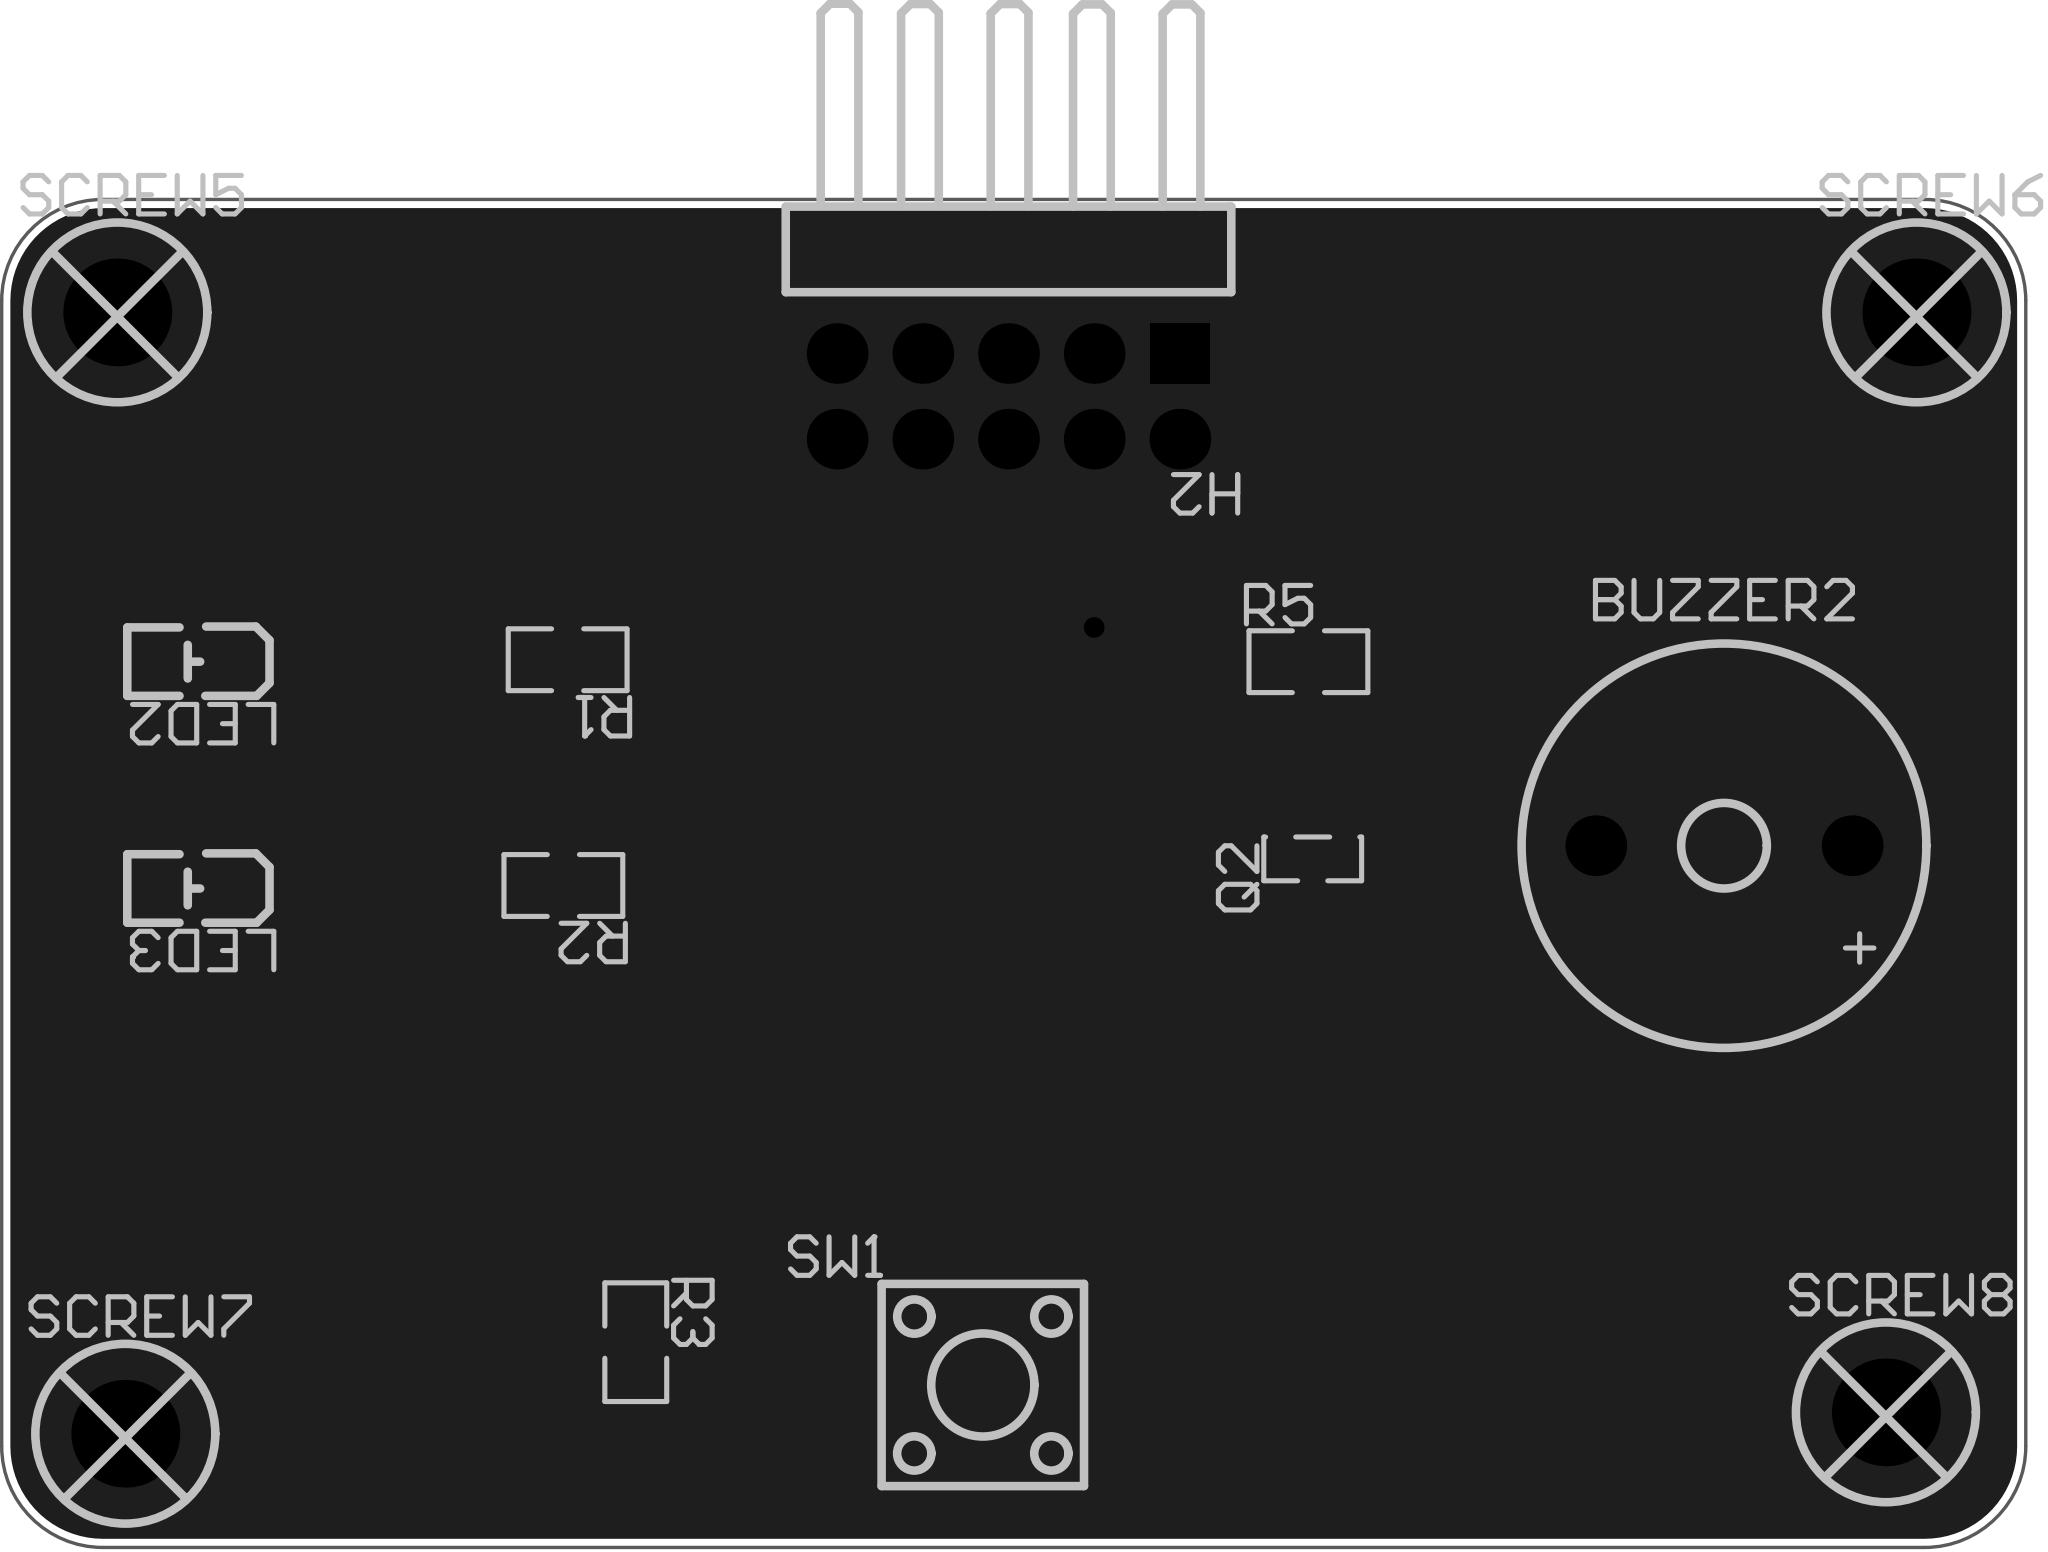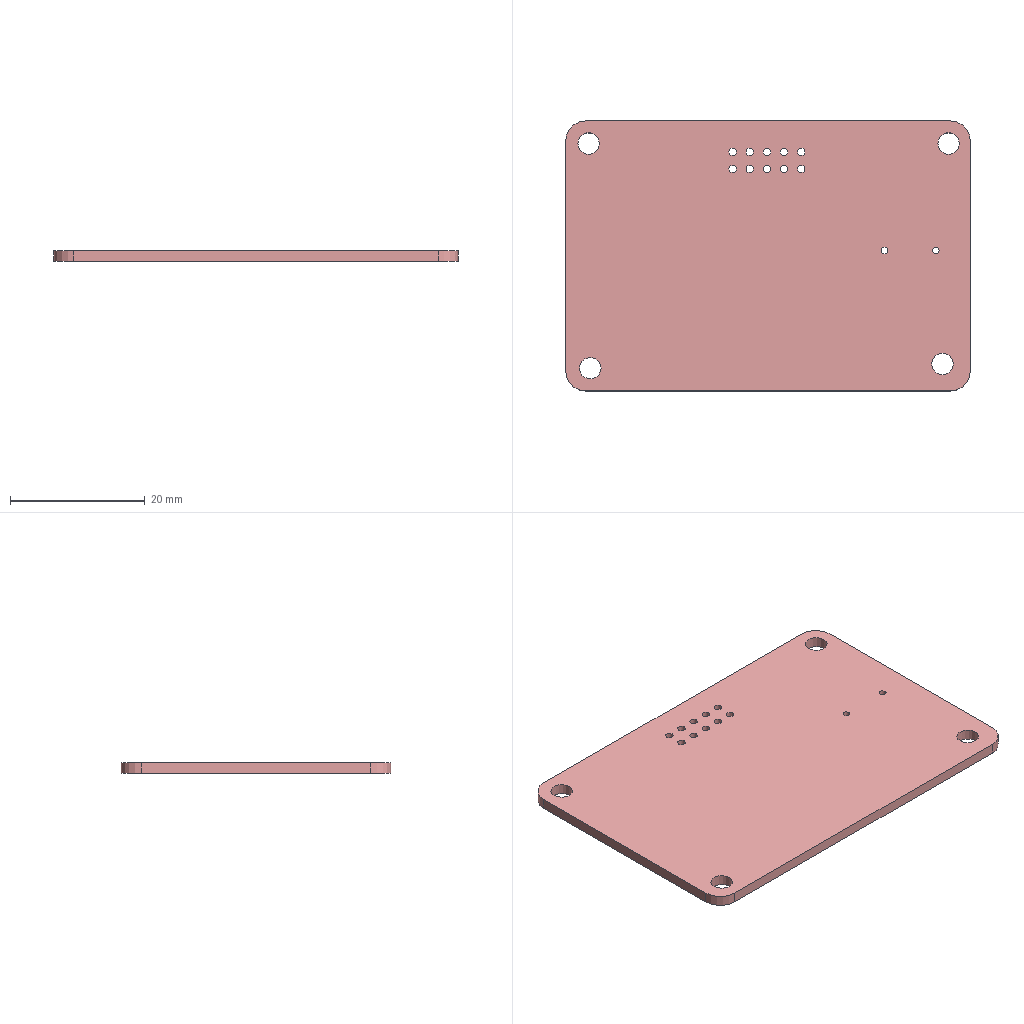Circuit board layout | Altium Designer | box 60 x 40 x 1.6 mm
Layer stack:
# Altium Designer layer stack of  (unit mm; dielectric type: 0 none, 1 core, 2 prepreg, 3 surface material)
index,name,kind,layer,copper_thickness_mm,dielectric_type,dielectric_thickness_mm,dielectric_material,dielectric_constant
0,Top Paste Mask Layer,other,,,,,,
1,Top Silkscreen Layer,other,,,,,,
2,Top Solder Mask Layer,dielectric,,,3,0.01,,3.3
3,Top Layer,copper,Top Layer,0.035,,,,
4,Dielectric1,dielectric,,,3,1.51,FR4,4.5
5,Bottom Layer,copper,Bottom Layer,0.035,,,,
6,Bottom Solder Mask Layer,dielectric,,,3,0.01,,3.3
7,Bottom Silkscreen Layer,other,,,,,,
8,Bottom Paste Mask Layer,other,,,,,,
# drill layer pairs: low layer,high layer
drill_pair,Top Layer,Bottom Layer
Part placement:
Designator,Comment,Layer,Footprint,Center-X(mm),Center-Y(mm),Rotation
R3,4.7k,TopLayer,R0805,99.568,90.043,270
H2,PZ254R-12-10P,TopLayer,HDR-TH_10P-P2.54-H-M-R2-C5-S2.54,110.617,118.11,180
LED2,GL0805UR01,TopLayer,LED0805-R-RD_RED,86.487,110.236,180
LED3,GL0805UR01,TopLayer,LED0805-R-RD_RED,86.487,103.505,180
Q2,S8050,TopLayer,SOT-23-3_L2.9-W1.3-P1.90-LS2.3-BR,119.634,104.394,90
R1,1k,TopLayer,R0805,97.548,110.294,180
R2,1k,TopLayer,R0805,97.421,103.595,180
R5,1k,TopLayer,R0805,119.507,110.236,0
SW1,KH-6X6X5H-STM,TopLayer,SW-SMD_4P-L6.0-W6.0-P4.50-LS9.0_H5.0,109.855,88.773,0
BUZZER2,2.4kHZ,TopLayer,BUZ-TH_BD12.0-P7.60-D0.6-FD,131.826,104.775,180
SCREW5,,TopLayer,M3螺丝,84.198,120.6,0
SCREW6,,TopLayer,M3螺丝,137.53,120.6,0
SCREW7,,TopLayer,M3螺丝,84.436,87.326,0
SCREW8,,TopLayer,M3螺丝,136.625,87.962,0
Pad and via stacks:
# Altium Designer via and pad stacks of  (unit mm). Each distinct definition once, with the count of objects using it.
# via: kind,start_layer,end_layer,hole_mm,diameter_mm,mode(0 simple;1 top-mid-bottom;2 full stack),diameter_per_layer,count,example_net
# pad: kind,layer,hole_mm,hole_type(0 round;1 square;2 slot),plating,top_size,top_shape(1 round;2 rect;3 octagon;9 rounded rect),mid_size,bottom_size,mode,footprint,size_per_layer,count,example
pad,Top Layer,0,0,plated,1.133x1.377,2,1.133x1.377,1.133x1.377,0,R0805,,8,R3.2
pad,Top Layer,0,0,plated,1x1.399,2,1x1.399,1x1.399,0,LED0805-R-RD_RED,,4,LED2.2
pad,Top Layer,0,0,plated,1.07x0.532,2,1.07x0.532,1.07x0.532,0,SOT-23-3_L2.9-W1.3-P1.90-LS2.3-BR,,3,Q2.3
pad,Top Layer,0,0,plated,2.3x1.5,2,2.3x1.5,2.3x1.5,0,SW-SMD_4P-L6.0-W6.0-P4.50-LS9.0_H5.0,,4,SW1.1
pad,Multi-Layer,1.1,0,plated,1.778x1.8,2,1.778x1.8,1.778x1.8,0,HDR-TH_10P-P2.54-H-M-R2-C5-S2.54,,1,H2.1
pad,Multi-Layer,1.1,0,plated,1.8x1.8,1,1.8x1.8,1.8x1.8,0,HDR-TH_10P-P2.54-H-M-R2-C5-S2.54,,9,H2.2
pad,Multi-Layer,1.001,0,plated,1.801x1.801,1,1.801x1.801,1.801x1.801,0,BUZ-TH_BD12.0-P7.60-D0.6-FD,,2,BUZZER2.2
pad,Multi-Layer,3.2,0,plated,3.2x3.2,1,3.2x3.2,3.2x3.2,0,M3\u00C2\u00DD\u00CB\u00BF,,4,SCREW5.1
via,Top Layer,Bottom Layer,0.3048,0.61,0,,1,GND
Copper pours:
name,layer,net,type(0 solid;1 hatched;2 none)
Top Layer-GND,Top Layer,GND,0
Design rules, without the lines most boards share:
# Altium Designer design rules of  (exported by Altium Designer, unit mm)
# columns: name | kind | enabled | priority | scope1 | scope2 | descriptor | typed fields (field=value)
copperRegion_Top Layer | 20 | enabled | 1 | (OnLayer('Top Layer')) | All | Polygon Connect Rule(Relief Connect )(Conductor Width=10mil) (Relief Angle=90 Angle) (Entries=4) (Air Gap Width=10mil) ((OnLayer('Top Layer'))),(All) | connect_style(0=relief,1=direct,2=none)=0 relief_conductor_width=0.254 relief_entries=4
copperRegion_Bottom Layer | 20 | enabled | 2 | (OnLayer('Bottom Layer')) | All | Polygon Connect Rule(Relief Connect )(Conductor Width=10mil) (Relief Angle=90 Angle) (Entries=4) (Air Gap Width=10mil) ((OnLayer('Bottom Layer'))),(All) | connect_style(0=relief,1=direct,2=none)=0 relief_conductor_width=0.254 relief_entries=4
copperRegion | 20 | enabled | 3 | All | All | Polygon Connect Rule(Direct Connect )(Conductor Width=10mil) (Relief Angle=90 Angle) (Entries=4) (Air Gap Width=10mil) (All),(All) | connect_style(0=relief,1=direct,2=none)=1 relief_conductor_width=0.254 relief_entries=4